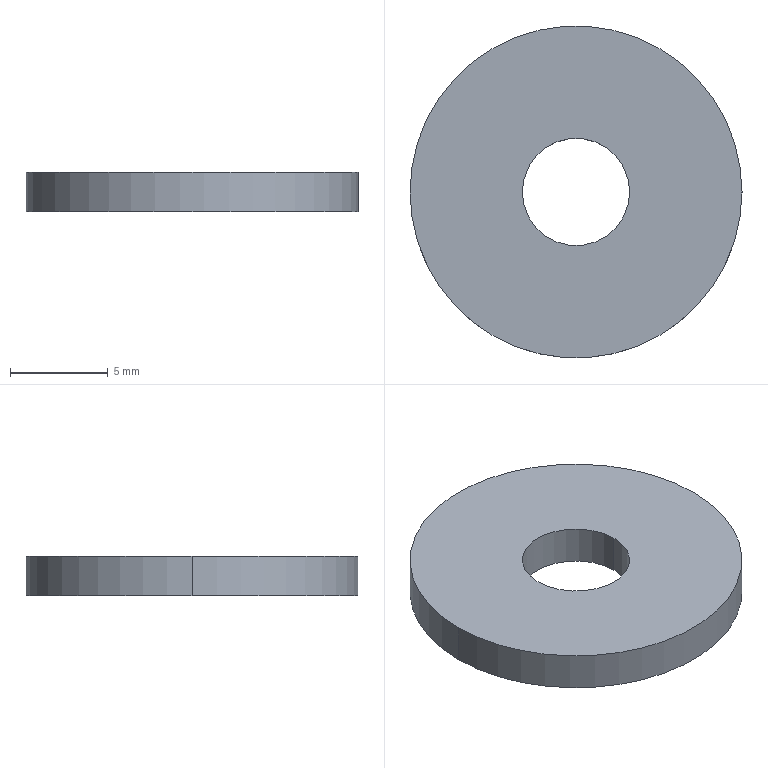Part | STEP file | MT-COMBO-119-S025 | 1 solid | 6 faces | box 17 x 17 x 2 mm | volume 406.444 mm3 | cylinder 4 | plane 2 | commonest cylinder face diameters 5.5 x2 17 x2
STEP:
#1=CARTESIAN_POINT('',(-2.75,0.,2.));
#2=VERTEX_POINT('',#1);
#3=CARTESIAN_POINT('',(2.75,0.,2.));
#4=VERTEX_POINT('',#3);
#5=CARTESIAN_POINT('',(0.,0.,2.));
#6=DIRECTION('',(0.,0.,1.));
#7=DIRECTION('',(1.,0.,0.));
#8=AXIS2_PLACEMENT_3D('',#5,#6,#7);
#9=CIRCLE('',#8,2.75);
#10=EDGE_CURVE('',#2,#4,#9,.T.);
#11=ORIENTED_EDGE('',*,*,#10,.T.);
#12=CARTESIAN_POINT('',(2.75,0.,0.));
#13=VERTEX_POINT('',#12);
#14=CARTESIAN_POINT('',(2.75,0.,2.));
#15=DIRECTION('',(0.,0.,-1.));
#16=VECTOR('',#15,1000.);
#17=LINE('',#14,#16);
#18=EDGE_CURVE('',#4,#13,#17,.T.);
#19=ORIENTED_EDGE('',*,*,#18,.T.);
#20=CARTESIAN_POINT('',(-2.75,0.,0.));
#21=VERTEX_POINT('',#20);
#22=CARTESIAN_POINT('',(0.,0.,0.));
#23=DIRECTION('',(0.,0.,1.));
#24=DIRECTION('',(1.,0.,0.));
#25=AXIS2_PLACEMENT_3D('',#22,#23,#24);
#26=CIRCLE('',#25,2.75);
#27=EDGE_CURVE('',#21,#13,#26,.T.);
#28=ORIENTED_EDGE('',*,*,#27,.F.);
#29=CARTESIAN_POINT('',(-2.75,0.,2.));
#30=DIRECTION('',(0.,0.,-1.));
#31=VECTOR('',#30,1000.);
#32=LINE('',#29,#31);
#33=EDGE_CURVE('',#2,#21,#32,.T.);
#34=ORIENTED_EDGE('',*,*,#33,.F.);
#35=EDGE_LOOP('',(#11,#19,#28,#34));
#36=FACE_OUTER_BOUND('',#35,.T.);
#37=CARTESIAN_POINT('',(0.,0.,2.));
#38=DIRECTION('',(0.,0.,-1.));
#39=DIRECTION('',(-1.,0.,0.));
#40=AXIS2_PLACEMENT_3D('',#37,#38,#39);
#41=CYLINDRICAL_SURFACE('',#40,2.75);
#42=ADVANCED_FACE('',(#36),#41,.F.);
#43=CARTESIAN_POINT('',(8.5,0.,2.));
#44=VERTEX_POINT('',#43);
#45=CARTESIAN_POINT('',(-8.5,0.,2.));
#46=VERTEX_POINT('',#45);
#47=CARTESIAN_POINT('',(0.,0.,2.));
#48=DIRECTION('',(0.,0.,1.));
#49=DIRECTION('',(1.,0.,0.));
#50=AXIS2_PLACEMENT_3D('',#47,#48,#49);
#51=CIRCLE('',#50,8.5);
#52=EDGE_CURVE('',#44,#46,#51,.T.);
#53=ORIENTED_EDGE('',*,*,#52,.F.);
#54=CARTESIAN_POINT('',(8.5,0.,0.));
#55=VERTEX_POINT('',#54);
#56=CARTESIAN_POINT('',(8.5,0.,2.));
#57=DIRECTION('',(0.,0.,-1.));
#58=VECTOR('',#57,1000.);
#59=LINE('',#56,#58);
#60=EDGE_CURVE('',#44,#55,#59,.T.);
#61=ORIENTED_EDGE('',*,*,#60,.T.);
#62=CARTESIAN_POINT('',(-8.5,0.,0.));
#63=VERTEX_POINT('',#62);
#64=CARTESIAN_POINT('',(0.,0.,0.));
#65=DIRECTION('',(0.,0.,1.));
#66=DIRECTION('',(1.,0.,0.));
#67=AXIS2_PLACEMENT_3D('',#64,#65,#66);
#68=CIRCLE('',#67,8.5);
#69=EDGE_CURVE('',#55,#63,#68,.T.);
#70=ORIENTED_EDGE('',*,*,#69,.T.);
#71=CARTESIAN_POINT('',(-8.5,0.,2.));
#72=DIRECTION('',(0.,0.,-1.));
#73=VECTOR('',#72,1000.);
#74=LINE('',#71,#73);
#75=EDGE_CURVE('',#46,#63,#74,.T.);
#76=ORIENTED_EDGE('',*,*,#75,.F.);
#77=EDGE_LOOP('',(#53,#61,#70,#76));
#78=FACE_OUTER_BOUND('',#77,.T.);
#79=CARTESIAN_POINT('',(0.,0.,2.));
#80=DIRECTION('',(0.,0.,-1.));
#81=DIRECTION('',(-1.,0.,0.));
#82=AXIS2_PLACEMENT_3D('',#79,#80,#81);
#83=CYLINDRICAL_SURFACE('',#82,8.5);
#84=ADVANCED_FACE('',(#78),#83,.T.);
#85=CARTESIAN_POINT('',(0.,0.,2.));
#86=DIRECTION('',(0.,0.,1.));
#87=DIRECTION('',(1.,0.,0.));
#88=AXIS2_PLACEMENT_3D('',#85,#86,#87);
#89=CIRCLE('',#88,8.5);
#90=EDGE_CURVE('',#46,#44,#89,.T.);
#91=ORIENTED_EDGE('',*,*,#90,.T.);
#92=ORIENTED_EDGE('',*,*,#52,.T.);
#93=EDGE_LOOP('',(#91,#92));
#94=FACE_OUTER_BOUND('',#93,.T.);
#95=ORIENTED_EDGE('',*,*,#10,.F.);
#96=CARTESIAN_POINT('',(0.,0.,2.));
#97=DIRECTION('',(0.,0.,1.));
#98=DIRECTION('',(1.,0.,0.));
#99=AXIS2_PLACEMENT_3D('',#96,#97,#98);
#100=CIRCLE('',#99,2.75);
#101=EDGE_CURVE('',#4,#2,#100,.T.);
#102=ORIENTED_EDGE('',*,*,#101,.F.);
#103=EDGE_LOOP('',(#95,#102));
#104=FACE_BOUND('',#103,.T.);
#105=CARTESIAN_POINT('',(0.,0.,2.));
#106=DIRECTION('',(0.,0.,1.));
#107=DIRECTION('',(1.,0.,0.));
#108=AXIS2_PLACEMENT_3D('',#105,#106,#107);
#109=PLANE('',#108);
#110=ADVANCED_FACE('',(#94,#104),#109,.T.);
#111=CARTESIAN_POINT('',(0.,0.,0.));
#112=DIRECTION('',(0.,0.,1.));
#113=DIRECTION('',(1.,0.,0.));
#114=AXIS2_PLACEMENT_3D('',#111,#112,#113);
#115=CIRCLE('',#114,8.5);
#116=EDGE_CURVE('',#63,#55,#115,.T.);
#117=ORIENTED_EDGE('',*,*,#116,.F.);
#118=ORIENTED_EDGE('',*,*,#69,.F.);
#119=EDGE_LOOP('',(#117,#118));
#120=FACE_OUTER_BOUND('',#119,.T.);
#121=ORIENTED_EDGE('',*,*,#27,.T.);
#122=CARTESIAN_POINT('',(0.,0.,0.));
#123=DIRECTION('',(0.,0.,1.));
#124=DIRECTION('',(1.,0.,0.));
#125=AXIS2_PLACEMENT_3D('',#122,#123,#124);
#126=CIRCLE('',#125,2.75);
#127=EDGE_CURVE('',#13,#21,#126,.T.);
#128=ORIENTED_EDGE('',*,*,#127,.T.);
#129=EDGE_LOOP('',(#121,#128));
#130=FACE_BOUND('',#129,.T.);
#131=CARTESIAN_POINT('',(0.,0.,0.));
#132=DIRECTION('',(0.,0.,1.));
#133=DIRECTION('',(1.,0.,0.));
#134=AXIS2_PLACEMENT_3D('',#131,#132,#133);
#135=PLANE('',#134);
#136=ADVANCED_FACE('',(#120,#130),#135,.F.);
#137=ORIENTED_EDGE('',*,*,#60,.F.);
#138=ORIENTED_EDGE('',*,*,#90,.F.);
#139=ORIENTED_EDGE('',*,*,#75,.T.);
#140=ORIENTED_EDGE('',*,*,#116,.T.);
#141=EDGE_LOOP('',(#137,#138,#139,#140));
#142=FACE_OUTER_BOUND('',#141,.T.);
#143=CARTESIAN_POINT('',(0.,0.,2.));
#144=DIRECTION('',(0.,0.,-1.));
#145=DIRECTION('',(-1.,0.,0.));
#146=AXIS2_PLACEMENT_3D('',#143,#144,#145);
#147=CYLINDRICAL_SURFACE('',#146,8.5);
#148=ADVANCED_FACE('',(#142),#147,.T.);
#149=ORIENTED_EDGE('',*,*,#18,.F.);
#150=ORIENTED_EDGE('',*,*,#101,.T.);
#151=ORIENTED_EDGE('',*,*,#33,.T.);
#152=ORIENTED_EDGE('',*,*,#127,.F.);
#153=EDGE_LOOP('',(#149,#150,#151,#152));
#154=FACE_OUTER_BOUND('',#153,.T.);
#155=CARTESIAN_POINT('',(0.,0.,2.));
#156=DIRECTION('',(0.,0.,-1.));
#157=DIRECTION('',(-1.,0.,0.));
#158=AXIS2_PLACEMENT_3D('',#155,#156,#157);
#159=CYLINDRICAL_SURFACE('',#158,2.75);
#160=ADVANCED_FACE('',(#154),#159,.F.);
#161=CLOSED_SHELL('',(#42,#84,#110,#136,#148,#160));
#162=MANIFOLD_SOLID_BREP('',#161);
#163=CARTESIAN_POINT('',(0.,0.,0.));
#164=DIRECTION('',(0.,0.,1.));
#165=DIRECTION('',(1.,0.,0.));
#166=AXIS2_PLACEMENT_3D('',#163,#164,#165);
#167=(LENGTH_UNIT()NAMED_UNIT(*)SI_UNIT(.MILLI.,.METRE.));
#168=UNCERTAINTY_MEASURE_WITH_UNIT(LENGTH_MEASURE(0.00001),#167,'','');
#169=(NAMED_UNIT(*)PLANE_ANGLE_UNIT()SI_UNIT($,.RADIAN.));
#170=(NAMED_UNIT(*)SI_UNIT($,.STERADIAN.)SOLID_ANGLE_UNIT());
#171=(GEOMETRIC_REPRESENTATION_CONTEXT(3)GLOBAL_UNCERTAINTY_ASSIGNED_CONTEXT((#168))GLOBAL_UNIT_ASSIGNED_CONTEXT((#167,#169,#170))REPRESENTATION_CONTEXT('',''));
#172=ADVANCED_BREP_SHAPE_REPRESENTATION('',(#162,#166),#171);